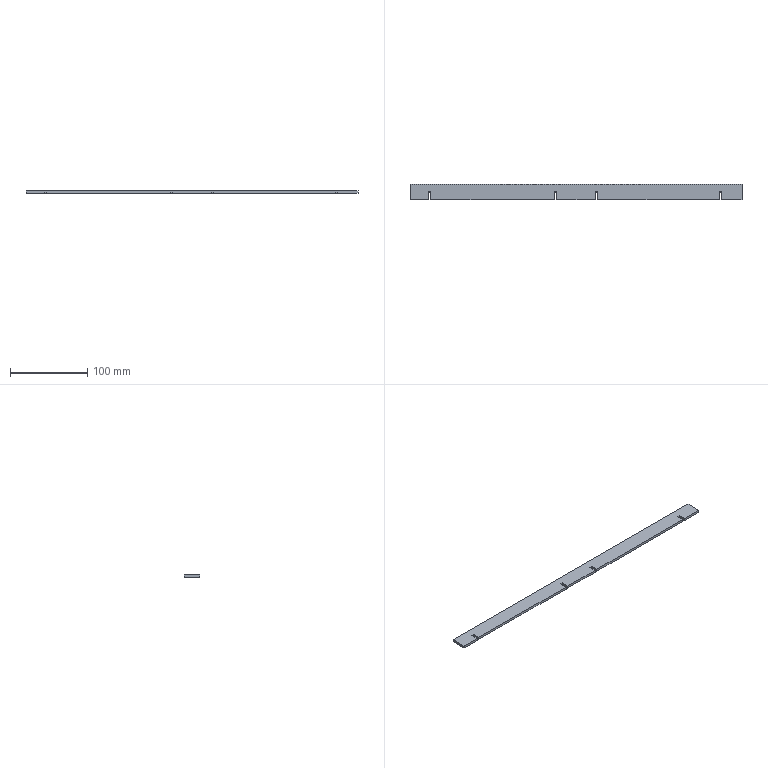Part | SolidWorks | features FlatPattern 1, SMBaseFlange 1, SheetMetal 1 | 1 solid | 22 faces | box 430 x 20 x 3.2 mm | volume 27110 mm3 | plane 22
STEP:
#1=CARTESIAN_POINT('',(-237.15,-378.4,0.));
#2=VERTEX_POINT('',#1);
#3=CARTESIAN_POINT('',(-237.15,-398.4,0.));
#4=VERTEX_POINT('',#3);
#5=CARTESIAN_POINT('',(-237.15,-398.4,0.));
#6=DIRECTION('',(0.,-1.,0.));
#7=VECTOR('',#6,1000.);
#8=LINE('',#5,#7);
#9=EDGE_CURVE('',#2,#4,#8,.T.);
#10=ORIENTED_EDGE('',*,*,#9,.F.);
#11=CARTESIAN_POINT('',(-237.15,-378.4,-3.2));
#12=VERTEX_POINT('',#11);
#13=CARTESIAN_POINT('',(-237.15,-378.4,-3.2));
#14=DIRECTION('',(0.,0.,1.));
#15=VECTOR('',#14,1000.);
#16=LINE('',#13,#15);
#17=EDGE_CURVE('',#12,#2,#16,.T.);
#18=ORIENTED_EDGE('',*,*,#17,.F.);
#19=CARTESIAN_POINT('',(-237.15,-398.4,-3.2));
#20=VERTEX_POINT('',#19);
#21=CARTESIAN_POINT('',(-237.15,-398.4,-3.2));
#22=DIRECTION('',(0.,-1.,0.));
#23=VECTOR('',#22,1000.);
#24=LINE('',#21,#23);
#25=EDGE_CURVE('',#12,#20,#24,.T.);
#26=ORIENTED_EDGE('',*,*,#25,.T.);
#27=CARTESIAN_POINT('',(-237.15,-398.4,-3.2));
#28=DIRECTION('',(0.,0.,1.));
#29=VECTOR('',#28,1000.);
#30=LINE('',#27,#29);
#31=EDGE_CURVE('',#20,#4,#30,.T.);
#32=ORIENTED_EDGE('',*,*,#31,.T.);
#33=EDGE_LOOP('',(#10,#18,#26,#32));
#34=FACE_OUTER_BOUND('',#33,.T.);
#35=CARTESIAN_POINT('',(-237.15,-398.4,-3.2));
#36=DIRECTION('',(-1.,0.,0.));
#37=DIRECTION('',(0.,0.,1.));
#38=AXIS2_PLACEMENT_3D('',#35,#36,#37);
#39=PLANE('',#38);
#40=ADVANCED_FACE('',(#34),#39,.T.);
#41=CARTESIAN_POINT('',(192.85,-378.4,0.));
#42=VERTEX_POINT('',#41);
#43=CARTESIAN_POINT('',(-237.15,-378.4,0.));
#44=DIRECTION('',(-1.,0.,0.));
#45=VECTOR('',#44,1000.);
#46=LINE('',#43,#45);
#47=EDGE_CURVE('',#42,#2,#46,.T.);
#48=ORIENTED_EDGE('',*,*,#47,.F.);
#49=CARTESIAN_POINT('',(192.85,-378.4,-3.2));
#50=VERTEX_POINT('',#49);
#51=CARTESIAN_POINT('',(192.85,-378.4,-3.2));
#52=DIRECTION('',(0.,0.,1.));
#53=VECTOR('',#52,1000.);
#54=LINE('',#51,#53);
#55=EDGE_CURVE('',#50,#42,#54,.T.);
#56=ORIENTED_EDGE('',*,*,#55,.F.);
#57=CARTESIAN_POINT('',(-237.15,-378.4,-3.2));
#58=DIRECTION('',(-1.,0.,0.));
#59=VECTOR('',#58,1000.);
#60=LINE('',#57,#59);
#61=EDGE_CURVE('',#50,#12,#60,.T.);
#62=ORIENTED_EDGE('',*,*,#61,.T.);
#63=ORIENTED_EDGE('',*,*,#17,.T.);
#64=EDGE_LOOP('',(#48,#56,#62,#63));
#65=FACE_OUTER_BOUND('',#64,.T.);
#66=CARTESIAN_POINT('',(-237.15,-378.4,-3.2));
#67=DIRECTION('',(0.,1.,0.));
#68=DIRECTION('',(0.,0.,1.));
#69=AXIS2_PLACEMENT_3D('',#66,#67,#68);
#70=PLANE('',#69);
#71=ADVANCED_FACE('',(#65),#70,.T.);
#72=CARTESIAN_POINT('',(192.85,-398.4,0.));
#73=VERTEX_POINT('',#72);
#74=CARTESIAN_POINT('',(192.85,-398.4,0.));
#75=DIRECTION('',(0.,1.,0.));
#76=VECTOR('',#75,1000.);
#77=LINE('',#74,#76);
#78=EDGE_CURVE('',#73,#42,#77,.T.);
#79=ORIENTED_EDGE('',*,*,#78,.F.);
#80=CARTESIAN_POINT('',(192.85,-398.4,-3.2));
#81=VERTEX_POINT('',#80);
#82=CARTESIAN_POINT('',(192.85,-398.4,-3.2));
#83=DIRECTION('',(0.,0.,1.));
#84=VECTOR('',#83,1000.);
#85=LINE('',#82,#84);
#86=EDGE_CURVE('',#81,#73,#85,.T.);
#87=ORIENTED_EDGE('',*,*,#86,.F.);
#88=CARTESIAN_POINT('',(192.85,-398.4,-3.2));
#89=DIRECTION('',(0.,1.,0.));
#90=VECTOR('',#89,1000.);
#91=LINE('',#88,#90);
#92=EDGE_CURVE('',#81,#50,#91,.T.);
#93=ORIENTED_EDGE('',*,*,#92,.T.);
#94=ORIENTED_EDGE('',*,*,#55,.T.);
#95=EDGE_LOOP('',(#79,#87,#93,#94));
#96=FACE_OUTER_BOUND('',#95,.T.);
#97=CARTESIAN_POINT('',(192.85,-398.4,-3.2));
#98=DIRECTION('',(1.,0.,0.));
#99=DIRECTION('',(0.,0.,-1.));
#100=AXIS2_PLACEMENT_3D('',#97,#98,#99);
#101=PLANE('',#100);
#102=ADVANCED_FACE('',(#96),#101,.T.);
#103=CARTESIAN_POINT('',(166.708,-398.4,0.));
#104=VERTEX_POINT('',#103);
#105=CARTESIAN_POINT('',(166.708,-398.4,0.));
#106=DIRECTION('',(1.,0.000000014,0.));
#107=VECTOR('',#106,1000.);
#108=LINE('',#105,#107);
#109=EDGE_CURVE('',#104,#73,#108,.T.);
#110=ORIENTED_EDGE('',*,*,#109,.F.);
#111=CARTESIAN_POINT('',(166.708,-398.4,-3.2));
#112=VERTEX_POINT('',#111);
#113=CARTESIAN_POINT('',(166.708,-398.4,-3.2));
#114=DIRECTION('',(0.,0.,1.));
#115=VECTOR('',#114,1000.);
#116=LINE('',#113,#115);
#117=EDGE_CURVE('',#112,#104,#116,.T.);
#118=ORIENTED_EDGE('',*,*,#117,.F.);
#119=CARTESIAN_POINT('',(166.708,-398.4,-3.2));
#120=DIRECTION('',(1.,0.000000014,0.));
#121=VECTOR('',#120,1000.);
#122=LINE('',#119,#121);
#123=EDGE_CURVE('',#112,#81,#122,.T.);
#124=ORIENTED_EDGE('',*,*,#123,.T.);
#125=ORIENTED_EDGE('',*,*,#86,.T.);
#126=EDGE_LOOP('',(#110,#118,#124,#125));
#127=FACE_OUTER_BOUND('',#126,.T.);
#128=CARTESIAN_POINT('',(166.708,-398.4,-3.2));
#129=DIRECTION('',(0.000000014,-1.,0.));
#130=DIRECTION('',(1.,0.000000014,0.));
#131=AXIS2_PLACEMENT_3D('',#128,#129,#130);
#132=PLANE('',#131);
#133=ADVANCED_FACE('',(#127),#132,.T.);
#134=CARTESIAN_POINT('',(166.708,-388.4,0.));
#135=VERTEX_POINT('',#134);
#136=CARTESIAN_POINT('',(166.708,-388.4,0.));
#137=DIRECTION('',(0.,-1.,0.));
#138=VECTOR('',#137,1000.);
#139=LINE('',#136,#138);
#140=EDGE_CURVE('',#135,#104,#139,.T.);
#141=ORIENTED_EDGE('',*,*,#140,.F.);
#142=CARTESIAN_POINT('',(166.708,-388.4,-3.2));
#143=VERTEX_POINT('',#142);
#144=CARTESIAN_POINT('',(166.708,-388.4,-3.2));
#145=DIRECTION('',(0.,0.,1.));
#146=VECTOR('',#145,1000.);
#147=LINE('',#144,#146);
#148=EDGE_CURVE('',#143,#135,#147,.T.);
#149=ORIENTED_EDGE('',*,*,#148,.F.);
#150=CARTESIAN_POINT('',(166.708,-388.4,-3.2));
#151=DIRECTION('',(0.,-1.,0.));
#152=VECTOR('',#151,1000.);
#153=LINE('',#150,#152);
#154=EDGE_CURVE('',#143,#112,#153,.T.);
#155=ORIENTED_EDGE('',*,*,#154,.T.);
#156=ORIENTED_EDGE('',*,*,#117,.T.);
#157=EDGE_LOOP('',(#141,#149,#155,#156));
#158=FACE_OUTER_BOUND('',#157,.T.);
#159=CARTESIAN_POINT('',(166.708,-388.4,-3.2));
#160=DIRECTION('',(-1.,0.,0.));
#161=DIRECTION('',(0.,0.,1.));
#162=AXIS2_PLACEMENT_3D('',#159,#160,#161);
#163=PLANE('',#162);
#164=ADVANCED_FACE('',(#158),#163,.T.);
#165=CARTESIAN_POINT('',(163.508,-388.4,0.));
#166=VERTEX_POINT('',#165);
#167=CARTESIAN_POINT('',(163.508,-388.4,0.));
#168=DIRECTION('',(1.,0.,0.));
#169=VECTOR('',#168,1000.);
#170=LINE('',#167,#169);
#171=EDGE_CURVE('',#166,#135,#170,.T.);
#172=ORIENTED_EDGE('',*,*,#171,.F.);
#173=CARTESIAN_POINT('',(163.508,-388.4,-3.2));
#174=VERTEX_POINT('',#173);
#175=CARTESIAN_POINT('',(163.508,-388.4,-3.2));
#176=DIRECTION('',(0.,0.,1.));
#177=VECTOR('',#176,1000.);
#178=LINE('',#175,#177);
#179=EDGE_CURVE('',#174,#166,#178,.T.);
#180=ORIENTED_EDGE('',*,*,#179,.F.);
#181=CARTESIAN_POINT('',(163.508,-388.4,-3.2));
#182=DIRECTION('',(1.,0.,0.));
#183=VECTOR('',#182,1000.);
#184=LINE('',#181,#183);
#185=EDGE_CURVE('',#174,#143,#184,.T.);
#186=ORIENTED_EDGE('',*,*,#185,.T.);
#187=ORIENTED_EDGE('',*,*,#148,.T.);
#188=EDGE_LOOP('',(#172,#180,#186,#187));
#189=FACE_OUTER_BOUND('',#188,.T.);
#190=CARTESIAN_POINT('',(163.508,-388.4,-3.2));
#191=DIRECTION('',(0.,-1.,0.));
#192=DIRECTION('',(0.,0.,-1.));
#193=AXIS2_PLACEMENT_3D('',#190,#191,#192);
#194=PLANE('',#193);
#195=ADVANCED_FACE('',(#189),#194,.T.);
#196=CARTESIAN_POINT('',(163.508,-398.4,0.));
#197=VERTEX_POINT('',#196);
#198=CARTESIAN_POINT('',(163.508,-398.4,0.));
#199=DIRECTION('',(0.,1.,0.));
#200=VECTOR('',#199,1000.);
#201=LINE('',#198,#200);
#202=EDGE_CURVE('',#197,#166,#201,.T.);
#203=ORIENTED_EDGE('',*,*,#202,.F.);
#204=CARTESIAN_POINT('',(163.508,-398.4,-3.2));
#205=VERTEX_POINT('',#204);
#206=CARTESIAN_POINT('',(163.508,-398.4,-3.2));
#207=DIRECTION('',(0.,0.,1.));
#208=VECTOR('',#207,1000.);
#209=LINE('',#206,#208);
#210=EDGE_CURVE('',#205,#197,#209,.T.);
#211=ORIENTED_EDGE('',*,*,#210,.F.);
#212=CARTESIAN_POINT('',(163.508,-398.4,-3.2));
#213=DIRECTION('',(0.,1.,0.));
#214=VECTOR('',#213,1000.);
#215=LINE('',#212,#214);
#216=EDGE_CURVE('',#205,#174,#215,.T.);
#217=ORIENTED_EDGE('',*,*,#216,.T.);
#218=ORIENTED_EDGE('',*,*,#179,.T.);
#219=EDGE_LOOP('',(#203,#211,#217,#218));
#220=FACE_OUTER_BOUND('',#219,.T.);
#221=CARTESIAN_POINT('',(163.508,-398.4,-3.2));
#222=DIRECTION('',(1.,0.,0.));
#223=DIRECTION('',(0.,0.,-1.));
#224=AXIS2_PLACEMENT_3D('',#221,#222,#223);
#225=PLANE('',#224);
#226=ADVANCED_FACE('',(#220),#225,.T.);
#227=CARTESIAN_POINT('',(6.05,-398.4,0.));
#228=VERTEX_POINT('',#227);
#229=CARTESIAN_POINT('',(6.05,-398.4,0.));
#230=DIRECTION('',(1.,0.,0.));
#231=VECTOR('',#230,1000.);
#232=LINE('',#229,#231);
#233=EDGE_CURVE('',#228,#197,#232,.T.);
#234=ORIENTED_EDGE('',*,*,#233,.F.);
#235=CARTESIAN_POINT('',(6.05,-398.4,-3.2));
#236=VERTEX_POINT('',#235);
#237=CARTESIAN_POINT('',(6.05,-398.4,-3.2));
#238=DIRECTION('',(0.,0.,1.));
#239=VECTOR('',#238,1000.);
#240=LINE('',#237,#239);
#241=EDGE_CURVE('',#236,#228,#240,.T.);
#242=ORIENTED_EDGE('',*,*,#241,.F.);
#243=CARTESIAN_POINT('',(6.05,-398.4,-3.2));
#244=DIRECTION('',(1.,0.,0.));
#245=VECTOR('',#244,1000.);
#246=LINE('',#243,#245);
#247=EDGE_CURVE('',#236,#205,#246,.T.);
#248=ORIENTED_EDGE('',*,*,#247,.T.);
#249=ORIENTED_EDGE('',*,*,#210,.T.);
#250=EDGE_LOOP('',(#234,#242,#248,#249));
#251=FACE_OUTER_BOUND('',#250,.T.);
#252=CARTESIAN_POINT('',(6.05,-398.4,-3.2));
#253=DIRECTION('',(0.,-1.,0.));
#254=DIRECTION('',(0.,0.,-1.));
#255=AXIS2_PLACEMENT_3D('',#252,#253,#254);
#256=PLANE('',#255);
#257=ADVANCED_FACE('',(#251),#256,.T.);
#258=CARTESIAN_POINT('',(6.05,-388.4,0.));
#259=VERTEX_POINT('',#258);
#260=CARTESIAN_POINT('',(6.05,-388.4,0.));
#261=DIRECTION('',(0.,-1.,0.));
#262=VECTOR('',#261,1000.);
#263=LINE('',#260,#262);
#264=EDGE_CURVE('',#259,#228,#263,.T.);
#265=ORIENTED_EDGE('',*,*,#264,.F.);
#266=CARTESIAN_POINT('',(6.05,-388.4,-3.2));
#267=VERTEX_POINT('',#266);
#268=CARTESIAN_POINT('',(6.05,-388.4,-3.2));
#269=DIRECTION('',(0.,0.,1.));
#270=VECTOR('',#269,1000.);
#271=LINE('',#268,#270);
#272=EDGE_CURVE('',#267,#259,#271,.T.);
#273=ORIENTED_EDGE('',*,*,#272,.F.);
#274=CARTESIAN_POINT('',(6.05,-388.4,-3.2));
#275=DIRECTION('',(0.,-1.,0.));
#276=VECTOR('',#275,1000.);
#277=LINE('',#274,#276);
#278=EDGE_CURVE('',#267,#236,#277,.T.);
#279=ORIENTED_EDGE('',*,*,#278,.T.);
#280=ORIENTED_EDGE('',*,*,#241,.T.);
#281=EDGE_LOOP('',(#265,#273,#279,#280));
#282=FACE_OUTER_BOUND('',#281,.T.);
#283=CARTESIAN_POINT('',(6.05,-388.4,-3.2));
#284=DIRECTION('',(-1.,0.,0.));
#285=DIRECTION('',(0.,-1.,0.));
#286=AXIS2_PLACEMENT_3D('',#283,#284,#285);
#287=PLANE('',#286);
#288=ADVANCED_FACE('',(#282),#287,.T.);
#289=CARTESIAN_POINT('',(2.85,-388.4,0.));
#290=VERTEX_POINT('',#289);
#291=CARTESIAN_POINT('',(2.85,-388.4,0.));
#292=DIRECTION('',(1.,0.,0.));
#293=VECTOR('',#292,1000.);
#294=LINE('',#291,#293);
#295=EDGE_CURVE('',#290,#259,#294,.T.);
#296=ORIENTED_EDGE('',*,*,#295,.F.);
#297=CARTESIAN_POINT('',(2.85,-388.4,-3.2));
#298=VERTEX_POINT('',#297);
#299=CARTESIAN_POINT('',(2.85,-388.4,-3.2));
#300=DIRECTION('',(0.,0.,1.));
#301=VECTOR('',#300,1000.);
#302=LINE('',#299,#301);
#303=EDGE_CURVE('',#298,#290,#302,.T.);
#304=ORIENTED_EDGE('',*,*,#303,.F.);
#305=CARTESIAN_POINT('',(2.85,-388.4,-3.2));
#306=DIRECTION('',(1.,0.,0.));
#307=VECTOR('',#306,1000.);
#308=LINE('',#305,#307);
#309=EDGE_CURVE('',#298,#267,#308,.T.);
#310=ORIENTED_EDGE('',*,*,#309,.T.);
#311=ORIENTED_EDGE('',*,*,#272,.T.);
#312=EDGE_LOOP('',(#296,#304,#310,#311));
#313=FACE_OUTER_BOUND('',#312,.T.);
#314=CARTESIAN_POINT('',(2.85,-388.4,-3.2));
#315=DIRECTION('',(0.,-1.,0.));
#316=DIRECTION('',(0.,0.,-1.));
#317=AXIS2_PLACEMENT_3D('',#314,#315,#316);
#318=PLANE('',#317);
#319=ADVANCED_FACE('',(#313),#318,.T.);
#320=CARTESIAN_POINT('',(2.85,-398.4,0.));
#321=VERTEX_POINT('',#320);
#322=CARTESIAN_POINT('',(2.85,-398.4,0.));
#323=DIRECTION('',(0.,1.,0.));
#324=VECTOR('',#323,1000.);
#325=LINE('',#322,#324);
#326=EDGE_CURVE('',#321,#290,#325,.T.);
#327=ORIENTED_EDGE('',*,*,#326,.F.);
#328=CARTESIAN_POINT('',(2.85,-398.4,-3.2));
#329=VERTEX_POINT('',#328);
#330=CARTESIAN_POINT('',(2.85,-398.4,-3.2));
#331=DIRECTION('',(0.,0.,1.));
#332=VECTOR('',#331,1000.);
#333=LINE('',#330,#332);
#334=EDGE_CURVE('',#329,#321,#333,.T.);
#335=ORIENTED_EDGE('',*,*,#334,.F.);
#336=CARTESIAN_POINT('',(2.85,-398.4,-3.2));
#337=DIRECTION('',(0.,1.,0.));
#338=VECTOR('',#337,1000.);
#339=LINE('',#336,#338);
#340=EDGE_CURVE('',#329,#298,#339,.T.);
#341=ORIENTED_EDGE('',*,*,#340,.T.);
#342=ORIENTED_EDGE('',*,*,#303,.T.);
#343=EDGE_LOOP('',(#327,#335,#341,#342));
#344=FACE_OUTER_BOUND('',#343,.T.);
#345=CARTESIAN_POINT('',(2.85,-398.4,-3.2));
#346=DIRECTION('',(1.,0.,0.));
#347=DIRECTION('',(0.,1.,0.));
#348=AXIS2_PLACEMENT_3D('',#345,#346,#347);
#349=PLANE('',#348);
#350=ADVANCED_FACE('',(#344),#349,.T.);
#351=CARTESIAN_POINT('',(-47.15,-398.4,0.));
#352=VERTEX_POINT('',#351);
#353=CARTESIAN_POINT('',(-47.15,-398.4,0.));
#354=DIRECTION('',(1.,0.,0.));
#355=VECTOR('',#354,1000.);
#356=LINE('',#353,#355);
#357=EDGE_CURVE('',#352,#321,#356,.T.);
#358=ORIENTED_EDGE('',*,*,#357,.F.);
#359=CARTESIAN_POINT('',(-47.15,-398.4,-3.2));
#360=VERTEX_POINT('',#359);
#361=CARTESIAN_POINT('',(-47.15,-398.4,-3.2));
#362=DIRECTION('',(0.,0.,1.));
#363=VECTOR('',#362,1000.);
#364=LINE('',#361,#363);
#365=EDGE_CURVE('',#360,#352,#364,.T.);
#366=ORIENTED_EDGE('',*,*,#365,.F.);
#367=CARTESIAN_POINT('',(-47.15,-398.4,-3.2));
#368=DIRECTION('',(1.,0.,0.));
#369=VECTOR('',#368,1000.);
#370=LINE('',#367,#369);
#371=EDGE_CURVE('',#360,#329,#370,.T.);
#372=ORIENTED_EDGE('',*,*,#371,.T.);
#373=ORIENTED_EDGE('',*,*,#334,.T.);
#374=EDGE_LOOP('',(#358,#366,#372,#373));
#375=FACE_OUTER_BOUND('',#374,.T.);
#376=CARTESIAN_POINT('',(-47.15,-398.4,-3.2));
#377=DIRECTION('',(0.,-1.,0.));
#378=DIRECTION('',(0.,0.,-1.));
#379=AXIS2_PLACEMENT_3D('',#376,#377,#378);
#380=PLANE('',#379);
#381=ADVANCED_FACE('',(#375),#380,.T.);
#382=CARTESIAN_POINT('',(-47.15,-388.4,0.));
#383=VERTEX_POINT('',#382);
#384=CARTESIAN_POINT('',(-47.15,-388.4,0.));
#385=DIRECTION('',(0.,-1.,0.));
#386=VECTOR('',#385,1000.);
#387=LINE('',#384,#386);
#388=EDGE_CURVE('',#383,#352,#387,.T.);
#389=ORIENTED_EDGE('',*,*,#388,.F.);
#390=CARTESIAN_POINT('',(-47.15,-388.4,-3.2));
#391=VERTEX_POINT('',#390);
#392=CARTESIAN_POINT('',(-47.15,-388.4,-3.2));
#393=DIRECTION('',(0.,0.,1.));
#394=VECTOR('',#393,1000.);
#395=LINE('',#392,#394);
#396=EDGE_CURVE('',#391,#383,#395,.T.);
#397=ORIENTED_EDGE('',*,*,#396,.F.);
#398=CARTESIAN_POINT('',(-47.15,-388.4,-3.2));
#399=DIRECTION('',(0.,-1.,0.));
#400=VECTOR('',#399,1000.);
#401=LINE('',#398,#400);
#402=EDGE_CURVE('',#391,#360,#401,.T.);
#403=ORIENTED_EDGE('',*,*,#402,.T.);
#404=ORIENTED_EDGE('',*,*,#365,.T.);
#405=EDGE_LOOP('',(#389,#397,#403,#404));
#406=FACE_OUTER_BOUND('',#405,.T.);
#407=CARTESIAN_POINT('',(-47.15,-388.4,-3.2));
#408=DIRECTION('',(-1.,0.,0.));
#409=DIRECTION('',(0.,-1.,0.));
#410=AXIS2_PLACEMENT_3D('',#407,#408,#409);
#411=PLANE('',#410);
#412=ADVANCED_FACE('',(#406),#411,.T.);
#413=CARTESIAN_POINT('',(-50.35,-388.4,0.));
#414=VERTEX_POINT('',#413);
#415=CARTESIAN_POINT('',(-50.35,-388.4,0.));
#416=DIRECTION('',(1.,0.,0.));
#417=VECTOR('',#416,1000.);
#418=LINE('',#415,#417);
#419=EDGE_CURVE('',#414,#383,#418,.T.);
#420=ORIENTED_EDGE('',*,*,#419,.F.);
#421=CARTESIAN_POINT('',(-50.35,-388.4,-3.2));
#422=VERTEX_POINT('',#421);
#423=CARTESIAN_POINT('',(-50.35,-388.4,-3.2));
#424=DIRECTION('',(0.,0.,1.));
#425=VECTOR('',#424,1000.);
#426=LINE('',#423,#425);
#427=EDGE_CURVE('',#422,#414,#426,.T.);
#428=ORIENTED_EDGE('',*,*,#427,.F.);
#429=CARTESIAN_POINT('',(-50.35,-388.4,-3.2));
#430=DIRECTION('',(1.,0.,0.));
#431=VECTOR('',#430,1000.);
#432=LINE('',#429,#431);
#433=EDGE_CURVE('',#422,#391,#432,.T.);
#434=ORIENTED_EDGE('',*,*,#433,.T.);
#435=ORIENTED_EDGE('',*,*,#396,.T.);
#436=EDGE_LOOP('',(#420,#428,#434,#435));
#437=FACE_OUTER_BOUND('',#436,.T.);
#438=CARTESIAN_POINT('',(-50.35,-388.4,-3.2));
#439=DIRECTION('',(0.,-1.,0.));
#440=DIRECTION('',(0.,0.,-1.));
#441=AXIS2_PLACEMENT_3D('',#438,#439,#440);
#442=PLANE('',#441);
#443=ADVANCED_FACE('',(#437),#442,.T.);
#444=CARTESIAN_POINT('',(-50.35,-398.4,0.));
#445=VERTEX_POINT('',#444);
#446=CARTESIAN_POINT('',(-50.35,-398.4,0.));
#447=DIRECTION('',(0.,1.,0.));
#448=VECTOR('',#447,1000.);
#449=LINE('',#446,#448);
#450=EDGE_CURVE('',#445,#414,#449,.T.);
#451=ORIENTED_EDGE('',*,*,#450,.F.);
#452=CARTESIAN_POINT('',(-50.35,-398.4,-3.2));
#453=VERTEX_POINT('',#452);
#454=CARTESIAN_POINT('',(-50.35,-398.4,-3.2));
#455=DIRECTION('',(0.,0.,1.));
#456=VECTOR('',#455,1000.);
#457=LINE('',#454,#456);
#458=EDGE_CURVE('',#453,#445,#457,.T.);
#459=ORIENTED_EDGE('',*,*,#458,.F.);
#460=CARTESIAN_POINT('',(-50.35,-398.4,-3.2));
#461=DIRECTION('',(0.,1.,0.));
#462=VECTOR('',#461,1000.);
#463=LINE('',#460,#462);
#464=EDGE_CURVE('',#453,#422,#463,.T.);
#465=ORIENTED_EDGE('',*,*,#464,.T.);
#466=ORIENTED_EDGE('',*,*,#427,.T.);
#467=EDGE_LOOP('',(#451,#459,#465,#466));
#468=FACE_OUTER_BOUND('',#467,.T.);
#469=CARTESIAN_POINT('',(-50.35,-398.4,-3.2));
#470=DIRECTION('',(1.,0.,0.));
#471=DIRECTION('',(0.,0.,-1.));
#472=AXIS2_PLACEMENT_3D('',#469,#470,#471);
#473=PLANE('',#472);
#474=ADVANCED_FACE('',(#468),#473,.T.);
#475=CARTESIAN_POINT('',(-210.092,-398.4,0.));
#476=VERTEX_POINT('',#475);
#477=CARTESIAN_POINT('',(-210.092,-398.4,0.));
#478=DIRECTION('',(1.,0.,0.));
#479=VECTOR('',#478,1000.);
#480=LINE('',#477,#479);
#481=EDGE_CURVE('',#476,#445,#480,.T.);
#482=ORIENTED_EDGE('',*,*,#481,.F.);
#483=CARTESIAN_POINT('',(-210.092,-398.4,-3.2));
#484=VERTEX_POINT('',#483);
#485=CARTESIAN_POINT('',(-210.092,-398.4,-3.2));
#486=DIRECTION('',(0.,0.,1.));
#487=VECTOR('',#486,1000.);
#488=LINE('',#485,#487);
#489=EDGE_CURVE('',#484,#476,#488,.T.);
#490=ORIENTED_EDGE('',*,*,#489,.F.);
#491=CARTESIAN_POINT('',(-210.092,-398.4,-3.2));
#492=DIRECTION('',(1.,0.,0.));
#493=VECTOR('',#492,1000.);
#494=LINE('',#491,#493);
#495=EDGE_CURVE('',#484,#453,#494,.T.);
#496=ORIENTED_EDGE('',*,*,#495,.T.);
#497=ORIENTED_EDGE('',*,*,#458,.T.);
#498=EDGE_LOOP('',(#482,#490,#496,#497));
#499=FACE_OUTER_BOUND('',#498,.T.);
#500=CARTESIAN_POINT('',(-210.092,-398.4,-3.2));
#501=DIRECTION('',(0.,-1.,0.));
#502=DIRECTION('',(0.,0.,-1.));
#503=AXIS2_PLACEMENT_3D('',#500,#501,#502);
#504=PLANE('',#503);
#505=ADVANCED_FACE('',(#499),#504,.T.);
#506=CARTESIAN_POINT('',(-210.092,-388.4,0.));
#507=VERTEX_POINT('',#506);
#508=CARTESIAN_POINT('',(-210.092,-388.4,0.));
#509=DIRECTION('',(0.,-1.,0.));
#510=VECTOR('',#509,1000.);
#511=LINE('',#508,#510);
#512=EDGE_CURVE('',#507,#476,#511,.T.);
#513=ORIENTED_EDGE('',*,*,#512,.F.);
#514=CARTESIAN_POINT('',(-210.092,-388.4,-3.2));
#515=VERTEX_POINT('',#514);
#516=CARTESIAN_POINT('',(-210.092,-388.4,-3.2));
#517=DIRECTION('',(0.,0.,1.));
#518=VECTOR('',#517,1000.);
#519=LINE('',#516,#518);
#520=EDGE_CURVE('',#515,#507,#519,.T.);
#521=ORIENTED_EDGE('',*,*,#520,.F.);
#522=CARTESIAN_POINT('',(-210.092,-388.4,-3.2));
#523=DIRECTION('',(0.,-1.,0.));
#524=VECTOR('',#523,1000.);
#525=LINE('',#522,#524);
#526=EDGE_CURVE('',#515,#484,#525,.T.);
#527=ORIENTED_EDGE('',*,*,#526,.T.);
#528=ORIENTED_EDGE('',*,*,#489,.T.);
#529=EDGE_LOOP('',(#513,#521,#527,#528));
#530=FACE_OUTER_BOUND('',#529,.T.);
#531=CARTESIAN_POINT('',(-210.092,-388.4,-3.2));
#532=DIRECTION('',(-1.,0.,0.));
#533=DIRECTION('',(0.,0.,1.));
#534=AXIS2_PLACEMENT_3D('',#531,#532,#533);
#535=PLANE('',#534);
#536=ADVANCED_FACE('',(#530),#535,.T.);
#537=CARTESIAN_POINT('',(-213.292,-388.4,0.));
#538=VERTEX_POINT('',#537);
#539=CARTESIAN_POINT('',(-213.292,-388.4,0.));
#540=DIRECTION('',(1.,0.,0.));
#541=VECTOR('',#540,1000.);
#542=LINE('',#539,#541);
#543=EDGE_CURVE('',#538,#507,#542,.T.);
#544=ORIENTED_EDGE('',*,*,#543,.F.);
#545=CARTESIAN_POINT('',(-213.292,-388.4,-3.2));
#546=VERTEX_POINT('',#545);
#547=CARTESIAN_POINT('',(-213.292,-388.4,-3.2));
#548=DIRECTION('',(0.,0.,1.));
#549=VECTOR('',#548,1000.);
#550=LINE('',#547,#549);
#551=EDGE_CURVE('',#546,#538,#550,.T.);
#552=ORIENTED_EDGE('',*,*,#551,.F.);
#553=CARTESIAN_POINT('',(-213.292,-388.4,-3.2));
#554=DIRECTION('',(1.,0.,0.));
#555=VECTOR('',#554,1000.);
#556=LINE('',#553,#555);
#557=EDGE_CURVE('',#546,#515,#556,.T.);
#558=ORIENTED_EDGE('',*,*,#557,.T.);
#559=ORIENTED_EDGE('',*,*,#520,.T.);
#560=EDGE_LOOP('',(#544,#552,#558,#559));
#561=FACE_OUTER_BOUND('',#560,.T.);
#562=CARTESIAN_POINT('',(-213.292,-388.4,-3.2));
#563=DIRECTION('',(0.,-1.,0.));
#564=DIRECTION('',(0.,0.,-1.));
#565=AXIS2_PLACEMENT_3D('',#562,#563,#564);
#566=PLANE('',#565);
#567=ADVANCED_FACE('',(#561),#566,.T.);
#568=CARTESIAN_POINT('',(-213.292,-398.4,0.));
#569=VERTEX_POINT('',#568);
#570=CARTESIAN_POINT('',(-213.292,-398.4,0.));
#571=DIRECTION('',(0.,1.,0.));
#572=VECTOR('',#571,1000.);
#573=LINE('',#570,#572);
#574=EDGE_CURVE('',#569,#538,#573,.T.);
#575=ORIENTED_EDGE('',*,*,#574,.F.);
#576=CARTESIAN_POINT('',(-213.292,-398.4,-3.2));
#577=VERTEX_POINT('',#576);
#578=CARTESIAN_POINT('',(-213.292,-398.4,-3.2));
#579=DIRECTION('',(0.,0.,1.));
#580=VECTOR('',#579,1000.);
#581=LINE('',#578,#580);
#582=EDGE_CURVE('',#577,#569,#581,.T.);
#583=ORIENTED_EDGE('',*,*,#582,.F.);
#584=CARTESIAN_POINT('',(-213.292,-398.4,-3.2));
#585=DIRECTION('',(0.,1.,0.));
#586=VECTOR('',#585,1000.);
#587=LINE('',#584,#586);
#588=EDGE_CURVE('',#577,#546,#587,.T.);
#589=ORIENTED_EDGE('',*,*,#588,.T.);
#590=ORIENTED_EDGE('',*,*,#551,.T.);
#591=EDGE_LOOP('',(#575,#583,#589,#590));
#592=FACE_OUTER_BOUND('',#591,.T.);
#593=CARTESIAN_POINT('',(-213.292,-398.4,-3.2));
#594=DIRECTION('',(1.,0.,0.));
#595=DIRECTION('',(0.,0.,-1.));
#596=AXIS2_PLACEMENT_3D('',#593,#594,#595);
#597=PLANE('',#596);
#598=ADVANCED_FACE('',(#592),#597,.T.);
#599=CARTESIAN_POINT('',(-237.15,-398.4,0.));
#600=DIRECTION('',(1.,-0.000000015,0.));
#601=VECTOR('',#600,1000.);
#602=LINE('',#599,#601);
#603=EDGE_CURVE('',#4,#569,#602,.T.);
#604=ORIENTED_EDGE('',*,*,#603,.F.);
#605=ORIENTED_EDGE('',*,*,#31,.F.);
#606=CARTESIAN_POINT('',(-237.15,-398.4,-3.2));
#607=DIRECTION('',(1.,-0.000000015,0.));
#608=VECTOR('',#607,1000.);
#609=LINE('',#606,#608);
#610=EDGE_CURVE('',#20,#577,#609,.T.);
#611=ORIENTED_EDGE('',*,*,#610,.T.);
#612=ORIENTED_EDGE('',*,*,#582,.T.);
#613=EDGE_LOOP('',(#604,#605,#611,#612));
#614=FACE_OUTER_BOUND('',#613,.T.);
#615=CARTESIAN_POINT('',(-237.15,-398.4,-3.2));
#616=DIRECTION('',(-0.000000015,-1.,0.));
#617=DIRECTION('',(1.,-0.000000015,0.));
#618=AXIS2_PLACEMENT_3D('',#615,#616,#617);
#619=PLANE('',#618);
#620=ADVANCED_FACE('',(#614),#619,.T.);
#621=ORIENTED_EDGE('',*,*,#25,.F.);
#622=ORIENTED_EDGE('',*,*,#61,.F.);
#623=ORIENTED_EDGE('',*,*,#92,.F.);
#624=ORIENTED_EDGE('',*,*,#123,.F.);
#625=ORIENTED_EDGE('',*,*,#154,.F.);
#626=ORIENTED_EDGE('',*,*,#185,.F.);
#627=ORIENTED_EDGE('',*,*,#216,.F.);
#628=ORIENTED_EDGE('',*,*,#247,.F.);
#629=ORIENTED_EDGE('',*,*,#278,.F.);
#630=ORIENTED_EDGE('',*,*,#309,.F.);
#631=ORIENTED_EDGE('',*,*,#340,.F.);
#632=ORIENTED_EDGE('',*,*,#371,.F.);
#633=ORIENTED_EDGE('',*,*,#402,.F.);
#634=ORIENTED_EDGE('',*,*,#433,.F.);
#635=ORIENTED_EDGE('',*,*,#464,.F.);
#636=ORIENTED_EDGE('',*,*,#495,.F.);
#637=ORIENTED_EDGE('',*,*,#526,.F.);
#638=ORIENTED_EDGE('',*,*,#557,.F.);
#639=ORIENTED_EDGE('',*,*,#588,.F.);
#640=ORIENTED_EDGE('',*,*,#610,.F.);
#641=EDGE_LOOP('',(#621,#622,#623,#624,#625,#626,#627,#628,#629,#630,#631,#632,#633,#634,#635,#636,#637,#638,#639,#640));
#642=FACE_OUTER_BOUND('',#641,.T.);
#643=CARTESIAN_POINT('',(0.,0.,-3.2));
#644=DIRECTION('',(0.,0.,-1.));
#645=DIRECTION('',(-1.,0.,0.));
#646=AXIS2_PLACEMENT_3D('',#643,#644,#645);
#647=PLANE('',#646);
#648=ADVANCED_FACE('',(#642),#647,.T.);
#649=ORIENTED_EDGE('',*,*,#9,.T.);
#650=ORIENTED_EDGE('',*,*,#603,.T.);
#651=ORIENTED_EDGE('',*,*,#574,.T.);
#652=ORIENTED_EDGE('',*,*,#543,.T.);
#653=ORIENTED_EDGE('',*,*,#512,.T.);
#654=ORIENTED_EDGE('',*,*,#481,.T.);
#655=ORIENTED_EDGE('',*,*,#450,.T.);
#656=ORIENTED_EDGE('',*,*,#419,.T.);
#657=ORIENTED_EDGE('',*,*,#388,.T.);
#658=ORIENTED_EDGE('',*,*,#357,.T.);
#659=ORIENTED_EDGE('',*,*,#326,.T.);
#660=ORIENTED_EDGE('',*,*,#295,.T.);
#661=ORIENTED_EDGE('',*,*,#264,.T.);
#662=ORIENTED_EDGE('',*,*,#233,.T.);
#663=ORIENTED_EDGE('',*,*,#202,.T.);
#664=ORIENTED_EDGE('',*,*,#171,.T.);
#665=ORIENTED_EDGE('',*,*,#140,.T.);
#666=ORIENTED_EDGE('',*,*,#109,.T.);
#667=ORIENTED_EDGE('',*,*,#78,.T.);
#668=ORIENTED_EDGE('',*,*,#47,.T.);
#669=EDGE_LOOP('',(#649,#650,#651,#652,#653,#654,#655,#656,#657,#658,#659,#660,#661,#662,#663,#664,#665,#666,#667,#668));
#670=FACE_OUTER_BOUND('',#669,.T.);
#671=CARTESIAN_POINT('',(0.,0.,0.));
#672=DIRECTION('',(0.,0.,-1.));
#673=DIRECTION('',(-1.,0.,0.));
#674=AXIS2_PLACEMENT_3D('',#671,#672,#673);
#675=PLANE('',#674);
#676=ADVANCED_FACE('',(#670),#675,.F.);
#677=CLOSED_SHELL('',(#40,#71,#102,#133,#164,#195,#226,#257,#288,#319,#350,#381,#412,#443,#474,#505,#536,#567,#598,#620,#648,#676));
#678=MANIFOLD_SOLID_BREP('',#677);
#679=CARTESIAN_POINT('',(0.,0.,0.));
#680=DIRECTION('',(0.,0.,1.));
#681=DIRECTION('',(1.,0.,0.));
#682=AXIS2_PLACEMENT_3D('',#679,#680,#681);
#683=(LENGTH_UNIT()NAMED_UNIT(*)SI_UNIT(.MILLI.,.METRE.));
#684=UNCERTAINTY_MEASURE_WITH_UNIT(LENGTH_MEASURE(0.00001),#683,'','');
#685=(NAMED_UNIT(*)PLANE_ANGLE_UNIT()SI_UNIT($,.RADIAN.));
#686=(NAMED_UNIT(*)SI_UNIT($,.STERADIAN.)SOLID_ANGLE_UNIT());
#687=(GEOMETRIC_REPRESENTATION_CONTEXT(3)GLOBAL_UNCERTAINTY_ASSIGNED_CONTEXT((#684))GLOBAL_UNIT_ASSIGNED_CONTEXT((#683,#685,#686))REPRESENTATION_CONTEXT('',''));
#688=ADVANCED_BREP_SHAPE_REPRESENTATION('',(#678,#682),#687);